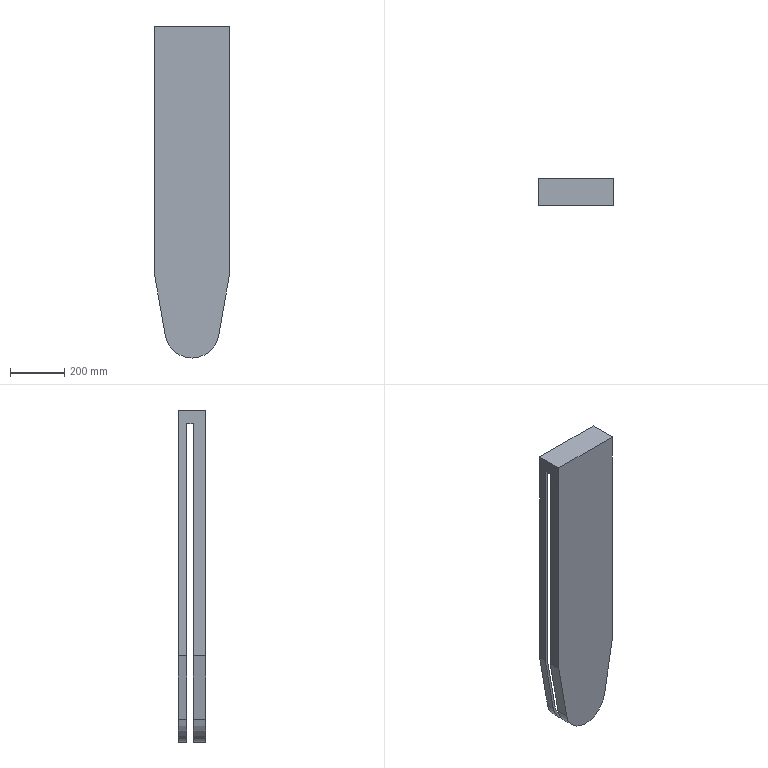Part | SolidWorks | 1 solid | 29 faces | box 280 x 100 x 1224 mm | volume 5139884 mm3 | plane 21 | cylinder 8 | commonest cylinder face diameters 180 x4 200 x4
STEP:
#1=CARTESIAN_POINT('',(88.633,45.,-1139.751));
#2=VERTEX_POINT('',#1);
#3=CARTESIAN_POINT('',(0.,45.,-1214.123));
#4=VERTEX_POINT('',#3);
#5=CARTESIAN_POINT('',(0.,45.,-1124.123));
#6=DIRECTION('',(0.,1.,0.));
#7=DIRECTION('',(0.,0.,-1.));
#8=AXIS2_PLACEMENT_3D('',#5,#6,#7);
#9=CIRCLE('',#8,90.);
#10=EDGE_CURVE('',#2,#4,#9,.T.);
#11=ORIENTED_EDGE('',*,*,#10,.T.);
#12=CARTESIAN_POINT('',(0.,10.,-1214.123));
#13=VERTEX_POINT('',#12);
#14=CARTESIAN_POINT('',(0.,100.,-1214.123));
#15=DIRECTION('',(0.,-1.,0.));
#16=VECTOR('',#15,1000.);
#17=LINE('',#14,#16);
#18=EDGE_CURVE('',#4,#13,#17,.T.);
#19=ORIENTED_EDGE('',*,*,#18,.T.);
#20=CARTESIAN_POINT('',(88.633,10.,-1139.751));
#21=VERTEX_POINT('',#20);
#22=CARTESIAN_POINT('',(0.,10.,-1124.123));
#23=DIRECTION('',(0.,-1.,0.));
#24=DIRECTION('',(0.,0.,-1.));
#25=AXIS2_PLACEMENT_3D('',#22,#23,#24);
#26=CIRCLE('',#25,90.);
#27=EDGE_CURVE('',#13,#21,#26,.T.);
#28=ORIENTED_EDGE('',*,*,#27,.T.);
#29=CARTESIAN_POINT('',(88.633,100.,-1139.751));
#30=DIRECTION('',(0.,1.,0.));
#31=VECTOR('',#30,1000.);
#32=LINE('',#29,#31);
#33=EDGE_CURVE('',#21,#2,#32,.T.);
#34=ORIENTED_EDGE('',*,*,#33,.T.);
#35=EDGE_LOOP('',(#11,#19,#28,#34));
#36=FACE_OUTER_BOUND('',#35,.T.);
#37=CARTESIAN_POINT('',(0.,100.,-1124.123));
#38=DIRECTION('',(0.,-1.,0.));
#39=DIRECTION('',(0.,0.,-1.));
#40=AXIS2_PLACEMENT_3D('',#37,#38,#39);
#41=CYLINDRICAL_SURFACE('',#40,90.);
#42=ADVANCED_FACE('',(#36),#41,.F.);
#43=CARTESIAN_POINT('',(0.,45.,-1224.123));
#44=VERTEX_POINT('',#43);
#45=CARTESIAN_POINT('',(-98.481,45.,-1141.488));
#46=VERTEX_POINT('',#45);
#47=CARTESIAN_POINT('',(0.,45.,-1124.123));
#48=DIRECTION('',(0.,1.,0.));
#49=DIRECTION('',(0.,0.,-1.));
#50=AXIS2_PLACEMENT_3D('',#47,#48,#49);
#51=CIRCLE('',#50,100.);
#52=EDGE_CURVE('',#44,#46,#51,.T.);
#53=ORIENTED_EDGE('',*,*,#52,.F.);
#54=CARTESIAN_POINT('',(0.,0.,-1224.123));
#55=VERTEX_POINT('',#54);
#56=CARTESIAN_POINT('',(0.,100.,-1224.123));
#57=DIRECTION('',(0.,-1.,0.));
#58=VECTOR('',#57,1000.);
#59=LINE('',#56,#58);
#60=EDGE_CURVE('',#44,#55,#59,.T.);
#61=ORIENTED_EDGE('',*,*,#60,.T.);
#62=CARTESIAN_POINT('',(-98.481,0.,-1141.488));
#63=VERTEX_POINT('',#62);
#64=CARTESIAN_POINT('',(0.,0.,-1124.123));
#65=DIRECTION('',(0.,-1.,0.));
#66=DIRECTION('',(0.,0.,-1.));
#67=AXIS2_PLACEMENT_3D('',#64,#65,#66);
#68=CIRCLE('',#67,100.);
#69=EDGE_CURVE('',#63,#55,#68,.T.);
#70=ORIENTED_EDGE('',*,*,#69,.F.);
#71=CARTESIAN_POINT('',(-98.481,100.,-1141.488));
#72=DIRECTION('',(0.,-1.,0.));
#73=VECTOR('',#72,1000.);
#74=LINE('',#71,#73);
#75=EDGE_CURVE('',#46,#63,#74,.T.);
#76=ORIENTED_EDGE('',*,*,#75,.F.);
#77=EDGE_LOOP('',(#53,#61,#70,#76));
#78=FACE_OUTER_BOUND('',#77,.T.);
#79=CARTESIAN_POINT('',(0.,100.,-1124.123));
#80=DIRECTION('',(0.,-1.,0.));
#81=DIRECTION('',(0.,0.,-1.));
#82=AXIS2_PLACEMENT_3D('',#79,#80,#81);
#83=CYLINDRICAL_SURFACE('',#82,100.);
#84=ADVANCED_FACE('',(#78),#83,.T.);
#85=CARTESIAN_POINT('',(88.633,100.,-1139.751));
#86=VERTEX_POINT('',#85);
#87=CARTESIAN_POINT('',(0.,100.,-1214.123));
#88=VERTEX_POINT('',#87);
#89=CARTESIAN_POINT('',(0.,100.,-1124.123));
#90=DIRECTION('',(0.,1.,0.));
#91=DIRECTION('',(0.,0.,-1.));
#92=AXIS2_PLACEMENT_3D('',#89,#90,#91);
#93=CIRCLE('',#92,90.);
#94=EDGE_CURVE('',#86,#88,#93,.T.);
#95=ORIENTED_EDGE('',*,*,#94,.T.);
#96=CARTESIAN_POINT('',(0.,70.,-1214.123));
#97=VERTEX_POINT('',#96);
#98=CARTESIAN_POINT('',(0.,100.,-1214.123));
#99=DIRECTION('',(0.,-1.,0.));
#100=VECTOR('',#99,1000.);
#101=LINE('',#98,#100);
#102=EDGE_CURVE('',#88,#97,#101,.T.);
#103=ORIENTED_EDGE('',*,*,#102,.T.);
#104=CARTESIAN_POINT('',(88.633,70.,-1139.751));
#105=VERTEX_POINT('',#104);
#106=CARTESIAN_POINT('',(0.,70.,-1124.123));
#107=DIRECTION('',(0.,-1.,0.));
#108=DIRECTION('',(0.,0.,1.));
#109=AXIS2_PLACEMENT_3D('',#106,#107,#108);
#110=CIRCLE('',#109,90.);
#111=EDGE_CURVE('',#97,#105,#110,.T.);
#112=ORIENTED_EDGE('',*,*,#111,.T.);
#113=CARTESIAN_POINT('',(88.633,100.,-1139.751));
#114=DIRECTION('',(0.,1.,0.));
#115=VECTOR('',#114,1000.);
#116=LINE('',#113,#115);
#117=EDGE_CURVE('',#105,#86,#116,.T.);
#118=ORIENTED_EDGE('',*,*,#117,.T.);
#119=EDGE_LOOP('',(#95,#103,#112,#118));
#120=FACE_OUTER_BOUND('',#119,.T.);
#121=CARTESIAN_POINT('',(0.,100.,-1124.123));
#122=DIRECTION('',(0.,-1.,0.));
#123=DIRECTION('',(0.,0.,-1.));
#124=AXIS2_PLACEMENT_3D('',#121,#122,#123);
#125=CYLINDRICAL_SURFACE('',#124,90.);
#126=ADVANCED_FACE('',(#120),#125,.F.);
#127=CARTESIAN_POINT('',(0.,100.,-1224.123));
#128=VERTEX_POINT('',#127);
#129=CARTESIAN_POINT('',(-98.481,100.,-1141.488));
#130=VERTEX_POINT('',#129);
#131=CARTESIAN_POINT('',(0.,100.,-1124.123));
#132=DIRECTION('',(0.,1.,0.));
#133=DIRECTION('',(0.,0.,-1.));
#134=AXIS2_PLACEMENT_3D('',#131,#132,#133);
#135=CIRCLE('',#134,100.);
#136=EDGE_CURVE('',#128,#130,#135,.T.);
#137=ORIENTED_EDGE('',*,*,#136,.F.);
#138=CARTESIAN_POINT('',(0.,70.,-1224.123));
#139=VERTEX_POINT('',#138);
#140=CARTESIAN_POINT('',(0.,100.,-1224.123));
#141=DIRECTION('',(0.,-1.,0.));
#142=VECTOR('',#141,1000.);
#143=LINE('',#140,#142);
#144=EDGE_CURVE('',#128,#139,#143,.T.);
#145=ORIENTED_EDGE('',*,*,#144,.T.);
#146=CARTESIAN_POINT('',(-98.481,70.,-1141.488));
#147=VERTEX_POINT('',#146);
#148=CARTESIAN_POINT('',(0.,70.,-1124.123));
#149=DIRECTION('',(0.,-1.,0.));
#150=DIRECTION('',(0.,0.,1.));
#151=AXIS2_PLACEMENT_3D('',#148,#149,#150);
#152=CIRCLE('',#151,100.);
#153=EDGE_CURVE('',#147,#139,#152,.T.);
#154=ORIENTED_EDGE('',*,*,#153,.F.);
#155=CARTESIAN_POINT('',(-98.481,100.,-1141.488));
#156=DIRECTION('',(0.,-1.,0.));
#157=VECTOR('',#156,1000.);
#158=LINE('',#155,#157);
#159=EDGE_CURVE('',#130,#147,#158,.T.);
#160=ORIENTED_EDGE('',*,*,#159,.F.);
#161=EDGE_LOOP('',(#137,#145,#154,#160));
#162=FACE_OUTER_BOUND('',#161,.T.);
#163=CARTESIAN_POINT('',(0.,100.,-1124.123));
#164=DIRECTION('',(0.,-1.,0.));
#165=DIRECTION('',(0.,0.,-1.));
#166=AXIS2_PLACEMENT_3D('',#163,#164,#165);
#167=CYLINDRICAL_SURFACE('',#166,100.);
#168=ADVANCED_FACE('',(#162),#167,.T.);
#169=ORIENTED_EDGE('',*,*,#159,.T.);
#170=CARTESIAN_POINT('',(-140.,70.,-906.021));
#171=VERTEX_POINT('',#170);
#172=CARTESIAN_POINT('',(0.,70.,-1700.));
#173=DIRECTION('',(-0.1736,0.,0.9848));
#174=VECTOR('',#173,1000.);
#175=LINE('',#172,#174);
#176=EDGE_CURVE('',#147,#171,#175,.T.);
#177=ORIENTED_EDGE('',*,*,#176,.T.);
#178=CARTESIAN_POINT('',(-140.,100.,-906.021));
#179=VERTEX_POINT('',#178);
#180=CARTESIAN_POINT('',(-140.,100.,-906.021));
#181=DIRECTION('',(0.,-1.,0.));
#182=VECTOR('',#181,1000.);
#183=LINE('',#180,#182);
#184=EDGE_CURVE('',#179,#171,#183,.T.);
#185=ORIENTED_EDGE('',*,*,#184,.F.);
#186=CARTESIAN_POINT('',(0.,100.,-1700.));
#187=DIRECTION('',(-0.1736,0.,0.9848));
#188=VECTOR('',#187,1000.);
#189=LINE('',#186,#188);
#190=EDGE_CURVE('',#130,#179,#189,.T.);
#191=ORIENTED_EDGE('',*,*,#190,.F.);
#192=EDGE_LOOP('',(#169,#177,#185,#191));
#193=FACE_OUTER_BOUND('',#192,.T.);
#194=CARTESIAN_POINT('',(0.,100.,-1700.));
#195=DIRECTION('',(0.9848,0.,0.1736));
#196=DIRECTION('',(0.1736,0.,-0.9848));
#197=AXIS2_PLACEMENT_3D('',#194,#195,#196);
#198=PLANE('',#197);
#199=ADVANCED_FACE('',(#193),#198,.F.);
#200=CARTESIAN_POINT('',(140.,100.,-906.021));
#201=VERTEX_POINT('',#200);
#202=CARTESIAN_POINT('',(140.,70.,-906.021));
#203=VERTEX_POINT('',#202);
#204=CARTESIAN_POINT('',(140.,100.,-906.021));
#205=DIRECTION('',(0.,-1.,0.));
#206=VECTOR('',#205,1000.);
#207=LINE('',#204,#206);
#208=EDGE_CURVE('',#201,#203,#207,.T.);
#209=ORIENTED_EDGE('',*,*,#208,.T.);
#210=CARTESIAN_POINT('',(98.481,70.,-1141.488));
#211=VERTEX_POINT('',#210);
#212=CARTESIAN_POINT('',(0.,70.,-1700.));
#213=DIRECTION('',(-0.1736,0.,-0.9848));
#214=VECTOR('',#213,1000.);
#215=LINE('',#212,#214);
#216=EDGE_CURVE('',#203,#211,#215,.T.);
#217=ORIENTED_EDGE('',*,*,#216,.T.);
#218=CARTESIAN_POINT('',(98.481,100.,-1141.488));
#219=VERTEX_POINT('',#218);
#220=CARTESIAN_POINT('',(98.481,100.,-1141.488));
#221=DIRECTION('',(0.,1.,0.));
#222=VECTOR('',#221,1000.);
#223=LINE('',#220,#222);
#224=EDGE_CURVE('',#211,#219,#223,.T.);
#225=ORIENTED_EDGE('',*,*,#224,.T.);
#226=CARTESIAN_POINT('',(0.,100.,-1700.));
#227=DIRECTION('',(-0.1736,0.,-0.9848));
#228=VECTOR('',#227,1000.);
#229=LINE('',#226,#228);
#230=EDGE_CURVE('',#201,#219,#229,.T.);
#231=ORIENTED_EDGE('',*,*,#230,.F.);
#232=EDGE_LOOP('',(#209,#217,#225,#231));
#233=FACE_OUTER_BOUND('',#232,.T.);
#234=CARTESIAN_POINT('',(0.,100.,-1700.));
#235=DIRECTION('',(-0.9848,0.,0.1736));
#236=DIRECTION('',(0.1736,0.,0.9848));
#237=AXIS2_PLACEMENT_3D('',#234,#235,#236);
#238=PLANE('',#237);
#239=ADVANCED_FACE('',(#233),#238,.F.);
#240=ORIENTED_EDGE('',*,*,#144,.F.);
#241=CARTESIAN_POINT('',(0.,100.,-1124.123));
#242=DIRECTION('',(0.,1.,0.));
#243=DIRECTION('',(0.,0.,-1.));
#244=AXIS2_PLACEMENT_3D('',#241,#242,#243);
#245=CIRCLE('',#244,100.);
#246=EDGE_CURVE('',#219,#128,#245,.T.);
#247=ORIENTED_EDGE('',*,*,#246,.F.);
#248=ORIENTED_EDGE('',*,*,#224,.F.);
#249=CARTESIAN_POINT('',(0.,70.,-1124.123));
#250=DIRECTION('',(0.,-1.,0.));
#251=DIRECTION('',(0.,0.,1.));
#252=AXIS2_PLACEMENT_3D('',#249,#250,#251);
#253=CIRCLE('',#252,100.);
#254=EDGE_CURVE('',#139,#211,#253,.T.);
#255=ORIENTED_EDGE('',*,*,#254,.F.);
#256=EDGE_LOOP('',(#240,#247,#248,#255));
#257=FACE_OUTER_BOUND('',#256,.T.);
#258=CARTESIAN_POINT('',(0.,100.,-1124.123));
#259=DIRECTION('',(0.,-1.,0.));
#260=DIRECTION('',(0.,0.,-1.));
#261=AXIS2_PLACEMENT_3D('',#258,#259,#260);
#262=CYLINDRICAL_SURFACE('',#261,100.);
#263=ADVANCED_FACE('',(#257),#262,.T.);
#264=CARTESIAN_POINT('',(-88.633,70.,-1139.751));
#265=VERTEX_POINT('',#264);
#266=CARTESIAN_POINT('',(-130.,70.,-905.146));
#267=VERTEX_POINT('',#266);
#268=CARTESIAN_POINT('',(9.848,70.,-1698.264));
#269=DIRECTION('',(-0.1736,0.,0.9848));
#270=VECTOR('',#269,1000.);
#271=LINE('',#268,#270);
#272=EDGE_CURVE('',#265,#267,#271,.T.);
#273=ORIENTED_EDGE('',*,*,#272,.F.);
#274=CARTESIAN_POINT('',(-88.633,100.,-1139.751));
#275=VERTEX_POINT('',#274);
#276=CARTESIAN_POINT('',(-88.633,100.,-1139.751));
#277=DIRECTION('',(0.,-1.,0.));
#278=VECTOR('',#277,1000.);
#279=LINE('',#276,#278);
#280=EDGE_CURVE('',#275,#265,#279,.T.);
#281=ORIENTED_EDGE('',*,*,#280,.F.);
#282=CARTESIAN_POINT('',(-130.,100.,-905.146));
#283=VERTEX_POINT('',#282);
#284=CARTESIAN_POINT('',(-280.869,100.,-49.525));
#285=DIRECTION('',(-0.1736,0.,0.9848));
#286=VECTOR('',#285,1000.);
#287=LINE('',#284,#286);
#288=EDGE_CURVE('',#275,#283,#287,.T.);
#289=ORIENTED_EDGE('',*,*,#288,.T.);
#290=CARTESIAN_POINT('',(-130.,100.,-905.146));
#291=DIRECTION('',(0.,-1.,0.));
#292=VECTOR('',#291,1000.);
#293=LINE('',#290,#292);
#294=EDGE_CURVE('',#283,#267,#293,.T.);
#295=ORIENTED_EDGE('',*,*,#294,.T.);
#296=EDGE_LOOP('',(#273,#281,#289,#295));
#297=FACE_OUTER_BOUND('',#296,.T.);
#298=CARTESIAN_POINT('',(9.848,100.,-1698.264));
#299=DIRECTION('',(0.9848,0.,0.1736));
#300=DIRECTION('',(0.1736,0.,-0.9848));
#301=AXIS2_PLACEMENT_3D('',#298,#299,#300);
#302=PLANE('',#301);
#303=ADVANCED_FACE('',(#297),#302,.T.);
#304=CARTESIAN_POINT('',(130.,70.,-905.146));
#305=VERTEX_POINT('',#304);
#306=CARTESIAN_POINT('',(-9.848,70.,-1698.264));
#307=DIRECTION('',(-0.1736,0.,-0.9848));
#308=VECTOR('',#307,1000.);
#309=LINE('',#306,#308);
#310=EDGE_CURVE('',#305,#105,#309,.T.);
#311=ORIENTED_EDGE('',*,*,#310,.F.);
#312=CARTESIAN_POINT('',(130.,100.,-905.146));
#313=VERTEX_POINT('',#312);
#314=CARTESIAN_POINT('',(130.,100.,-905.146));
#315=DIRECTION('',(0.,-1.,0.));
#316=VECTOR('',#315,1000.);
#317=LINE('',#314,#316);
#318=EDGE_CURVE('',#313,#305,#317,.T.);
#319=ORIENTED_EDGE('',*,*,#318,.F.);
#320=CARTESIAN_POINT('',(280.869,100.,-49.525));
#321=DIRECTION('',(-0.1736,0.,-0.9848));
#322=VECTOR('',#321,1000.);
#323=LINE('',#320,#322);
#324=EDGE_CURVE('',#313,#86,#323,.T.);
#325=ORIENTED_EDGE('',*,*,#324,.T.);
#326=ORIENTED_EDGE('',*,*,#117,.F.);
#327=EDGE_LOOP('',(#311,#319,#325,#326));
#328=FACE_OUTER_BOUND('',#327,.T.);
#329=CARTESIAN_POINT('',(-9.848,100.,-1698.264));
#330=DIRECTION('',(-0.9848,0.,0.1736));
#331=DIRECTION('',(0.1736,0.,0.9848));
#332=AXIS2_PLACEMENT_3D('',#329,#330,#331);
#333=PLANE('',#332);
#334=ADVANCED_FACE('',(#328),#333,.T.);
#335=ORIENTED_EDGE('',*,*,#102,.F.);
#336=CARTESIAN_POINT('',(0.,100.,-1124.123));
#337=DIRECTION('',(0.,1.,0.));
#338=DIRECTION('',(0.,0.,-1.));
#339=AXIS2_PLACEMENT_3D('',#336,#337,#338);
#340=CIRCLE('',#339,90.);
#341=EDGE_CURVE('',#88,#275,#340,.T.);
#342=ORIENTED_EDGE('',*,*,#341,.T.);
#343=ORIENTED_EDGE('',*,*,#280,.T.);
#344=CARTESIAN_POINT('',(0.,70.,-1124.123));
#345=DIRECTION('',(0.,-1.,0.));
#346=DIRECTION('',(0.,0.,1.));
#347=AXIS2_PLACEMENT_3D('',#344,#345,#346);
#348=CIRCLE('',#347,90.);
#349=EDGE_CURVE('',#265,#97,#348,.T.);
#350=ORIENTED_EDGE('',*,*,#349,.T.);
#351=EDGE_LOOP('',(#335,#342,#343,#350));
#352=FACE_OUTER_BOUND('',#351,.T.);
#353=CARTESIAN_POINT('',(0.,100.,-1124.123));
#354=DIRECTION('',(0.,-1.,0.));
#355=DIRECTION('',(0.,0.,-1.));
#356=AXIS2_PLACEMENT_3D('',#353,#354,#355);
#357=CYLINDRICAL_SURFACE('',#356,90.);
#358=ADVANCED_FACE('',(#352),#357,.F.);
#359=ORIENTED_EDGE('',*,*,#230,.T.);
#360=ORIENTED_EDGE('',*,*,#246,.T.);
#361=ORIENTED_EDGE('',*,*,#136,.T.);
#362=ORIENTED_EDGE('',*,*,#190,.T.);
#363=CARTESIAN_POINT('',(-140.,100.,0.));
#364=VERTEX_POINT('',#363);
#365=CARTESIAN_POINT('',(-140.,100.,-906.021));
#366=DIRECTION('',(0.,0.,1.));
#367=VECTOR('',#366,1000.);
#368=LINE('',#365,#367);
#369=EDGE_CURVE('',#179,#364,#368,.T.);
#370=ORIENTED_EDGE('',*,*,#369,.T.);
#371=CARTESIAN_POINT('',(140.,100.,0.));
#372=VERTEX_POINT('',#371);
#373=CARTESIAN_POINT('',(140.,100.,0.));
#374=DIRECTION('',(1.,0.,0.));
#375=VECTOR('',#374,1000.);
#376=LINE('',#373,#375);
#377=EDGE_CURVE('',#364,#372,#376,.T.);
#378=ORIENTED_EDGE('',*,*,#377,.T.);
#379=CARTESIAN_POINT('',(140.,100.,-906.021));
#380=DIRECTION('',(0.,0.,-1.));
#381=VECTOR('',#380,1000.);
#382=LINE('',#379,#381);
#383=EDGE_CURVE('',#372,#201,#382,.T.);
#384=ORIENTED_EDGE('',*,*,#383,.T.);
#385=EDGE_LOOP('',(#359,#360,#361,#362,#370,#378,#384));
#386=FACE_OUTER_BOUND('',#385,.T.);
#387=ORIENTED_EDGE('',*,*,#324,.F.);
#388=CARTESIAN_POINT('',(130.,100.,-10.));
#389=VERTEX_POINT('',#388);
#390=CARTESIAN_POINT('',(130.,100.,0.));
#391=DIRECTION('',(0.,0.,-1.));
#392=VECTOR('',#391,1000.);
#393=LINE('',#390,#392);
#394=EDGE_CURVE('',#389,#313,#393,.T.);
#395=ORIENTED_EDGE('',*,*,#394,.F.);
#396=CARTESIAN_POINT('',(-130.,100.,-10.));
#397=VERTEX_POINT('',#396);
#398=CARTESIAN_POINT('',(0.,100.,-10.));
#399=DIRECTION('',(1.,0.,0.));
#400=VECTOR('',#399,1000.);
#401=LINE('',#398,#400);
#402=EDGE_CURVE('',#397,#389,#401,.T.);
#403=ORIENTED_EDGE('',*,*,#402,.F.);
#404=CARTESIAN_POINT('',(-130.,100.,0.));
#405=DIRECTION('',(0.,0.,1.));
#406=VECTOR('',#405,1000.);
#407=LINE('',#404,#406);
#408=EDGE_CURVE('',#283,#397,#407,.T.);
#409=ORIENTED_EDGE('',*,*,#408,.F.);
#410=ORIENTED_EDGE('',*,*,#288,.F.);
#411=ORIENTED_EDGE('',*,*,#341,.F.);
#412=ORIENTED_EDGE('',*,*,#94,.F.);
#413=EDGE_LOOP('',(#387,#395,#403,#409,#410,#411,#412));
#414=FACE_BOUND('',#413,.T.);
#415=CARTESIAN_POINT('',(0.,100.,0.));
#416=DIRECTION('',(0.,-1.,0.));
#417=DIRECTION('',(0.,0.,-1.));
#418=AXIS2_PLACEMENT_3D('',#415,#416,#417);
#419=PLANE('',#418);
#420=ADVANCED_FACE('',(#386,#414),#419,.F.);
#421=CARTESIAN_POINT('',(-140.,45.,-906.021));
#422=VERTEX_POINT('',#421);
#423=CARTESIAN_POINT('',(-140.,0.,-906.021));
#424=VERTEX_POINT('',#423);
#425=CARTESIAN_POINT('',(-140.,100.,-906.021));
#426=DIRECTION('',(0.,-1.,0.));
#427=VECTOR('',#426,1000.);
#428=LINE('',#425,#427);
#429=EDGE_CURVE('',#422,#424,#428,.T.);
#430=ORIENTED_EDGE('',*,*,#429,.F.);
#431=CARTESIAN_POINT('',(0.,45.,-1700.));
#432=DIRECTION('',(0.1736,0.,-0.9848));
#433=VECTOR('',#432,1000.);
#434=LINE('',#431,#433);
#435=EDGE_CURVE('',#422,#46,#434,.T.);
#436=ORIENTED_EDGE('',*,*,#435,.T.);
#437=ORIENTED_EDGE('',*,*,#75,.T.);
#438=CARTESIAN_POINT('',(0.,0.,-1700.));
#439=DIRECTION('',(-0.1736,0.,0.9848));
#440=VECTOR('',#439,1000.);
#441=LINE('',#438,#440);
#442=EDGE_CURVE('',#63,#424,#441,.T.);
#443=ORIENTED_EDGE('',*,*,#442,.T.);
#444=EDGE_LOOP('',(#430,#436,#437,#443));
#445=FACE_OUTER_BOUND('',#444,.T.);
#446=CARTESIAN_POINT('',(0.,100.,-1700.));
#447=DIRECTION('',(0.9848,0.,0.1736));
#448=DIRECTION('',(0.1736,0.,-0.9848));
#449=AXIS2_PLACEMENT_3D('',#446,#447,#448);
#450=PLANE('',#449);
#451=ADVANCED_FACE('',(#445),#450,.F.);
#452=ORIENTED_EDGE('',*,*,#184,.T.);
#453=CARTESIAN_POINT('',(-140.,70.,-50.));
#454=VERTEX_POINT('',#453);
#455=CARTESIAN_POINT('',(-140.,70.,-1224.123));
#456=DIRECTION('',(0.,0.,-1.));
#457=VECTOR('',#456,1000.);
#458=LINE('',#455,#457);
#459=EDGE_CURVE('',#454,#171,#458,.T.);
#460=ORIENTED_EDGE('',*,*,#459,.F.);
#461=CARTESIAN_POINT('',(-140.,45.,-50.));
#462=VERTEX_POINT('',#461);
#463=CARTESIAN_POINT('',(-140.,70.,-50.));
#464=DIRECTION('',(0.,1.,0.));
#465=VECTOR('',#464,1000.);
#466=LINE('',#463,#465);
#467=EDGE_CURVE('',#462,#454,#466,.T.);
#468=ORIENTED_EDGE('',*,*,#467,.F.);
#469=CARTESIAN_POINT('',(-140.,45.,-1224.123));
#470=DIRECTION('',(0.,0.,1.));
#471=VECTOR('',#470,1000.);
#472=LINE('',#469,#471);
#473=EDGE_CURVE('',#422,#462,#472,.T.);
#474=ORIENTED_EDGE('',*,*,#473,.F.);
#475=ORIENTED_EDGE('',*,*,#429,.T.);
#476=CARTESIAN_POINT('',(-140.,0.,0.));
#477=VERTEX_POINT('',#476);
#478=CARTESIAN_POINT('',(-140.,0.,-906.021));
#479=DIRECTION('',(0.,0.,1.));
#480=VECTOR('',#479,1000.);
#481=LINE('',#478,#480);
#482=EDGE_CURVE('',#424,#477,#481,.T.);
#483=ORIENTED_EDGE('',*,*,#482,.T.);
#484=CARTESIAN_POINT('',(-140.,100.,0.));
#485=DIRECTION('',(0.,-1.,0.));
#486=VECTOR('',#485,1000.);
#487=LINE('',#484,#486);
#488=EDGE_CURVE('',#364,#477,#487,.T.);
#489=ORIENTED_EDGE('',*,*,#488,.F.);
#490=ORIENTED_EDGE('',*,*,#369,.F.);
#491=EDGE_LOOP('',(#452,#460,#468,#474,#475,#483,#489,#490));
#492=FACE_OUTER_BOUND('',#491,.T.);
#493=CARTESIAN_POINT('',(-140.,100.,-906.021));
#494=DIRECTION('',(1.,0.,0.));
#495=DIRECTION('',(0.,0.,-1.));
#496=AXIS2_PLACEMENT_3D('',#493,#494,#495);
#497=PLANE('',#496);
#498=ADVANCED_FACE('',(#492),#497,.F.);
#499=CARTESIAN_POINT('',(140.,0.,0.));
#500=VERTEX_POINT('',#499);
#501=CARTESIAN_POINT('',(140.,0.,0.));
#502=DIRECTION('',(1.,0.,0.));
#503=VECTOR('',#502,1000.);
#504=LINE('',#501,#503);
#505=EDGE_CURVE('',#477,#500,#504,.T.);
#506=ORIENTED_EDGE('',*,*,#505,.T.);
#507=CARTESIAN_POINT('',(140.,100.,0.));
#508=DIRECTION('',(0.,-1.,0.));
#509=VECTOR('',#508,1000.);
#510=LINE('',#507,#509);
#511=EDGE_CURVE('',#372,#500,#510,.T.);
#512=ORIENTED_EDGE('',*,*,#511,.F.);
#513=ORIENTED_EDGE('',*,*,#377,.F.);
#514=ORIENTED_EDGE('',*,*,#488,.T.);
#515=EDGE_LOOP('',(#506,#512,#513,#514));
#516=FACE_OUTER_BOUND('',#515,.T.);
#517=CARTESIAN_POINT('',(140.,100.,0.));
#518=DIRECTION('',(0.,0.,-1.));
#519=DIRECTION('',(-1.,0.,0.));
#520=AXIS2_PLACEMENT_3D('',#517,#518,#519);
#521=PLANE('',#520);
#522=ADVANCED_FACE('',(#516),#521,.F.);
#523=CARTESIAN_POINT('',(140.,45.,-50.));
#524=VERTEX_POINT('',#523);
#525=CARTESIAN_POINT('',(140.,70.,-50.));
#526=VERTEX_POINT('',#525);
#527=CARTESIAN_POINT('',(140.,100.,-50.));
#528=DIRECTION('',(0.,1.,0.));
#529=VECTOR('',#528,1000.);
#530=LINE('',#527,#529);
#531=EDGE_CURVE('',#524,#526,#530,.T.);
#532=ORIENTED_EDGE('',*,*,#531,.T.);
#533=CARTESIAN_POINT('',(140.,70.,-906.021));
#534=DIRECTION('',(0.,0.,-1.));
#535=VECTOR('',#534,1000.);
#536=LINE('',#533,#535);
#537=EDGE_CURVE('',#526,#203,#536,.T.);
#538=ORIENTED_EDGE('',*,*,#537,.T.);
#539=ORIENTED_EDGE('',*,*,#208,.F.);
#540=ORIENTED_EDGE('',*,*,#383,.F.);
#541=ORIENTED_EDGE('',*,*,#511,.T.);
#542=CARTESIAN_POINT('',(140.,0.,-906.021));
#543=VERTEX_POINT('',#542);
#544=CARTESIAN_POINT('',(140.,0.,-906.021));
#545=DIRECTION('',(0.,0.,-1.));
#546=VECTOR('',#545,1000.);
#547=LINE('',#544,#546);
#548=EDGE_CURVE('',#500,#543,#547,.T.);
#549=ORIENTED_EDGE('',*,*,#548,.T.);
#550=CARTESIAN_POINT('',(140.,45.,-906.021));
#551=VERTEX_POINT('',#550);
#552=CARTESIAN_POINT('',(140.,100.,-906.021));
#553=DIRECTION('',(0.,-1.,0.));
#554=VECTOR('',#553,1000.);
#555=LINE('',#552,#554);
#556=EDGE_CURVE('',#551,#543,#555,.T.);
#557=ORIENTED_EDGE('',*,*,#556,.F.);
#558=CARTESIAN_POINT('',(140.,45.,-906.021));
#559=DIRECTION('',(0.,0.,1.));
#560=VECTOR('',#559,1000.);
#561=LINE('',#558,#560);
#562=EDGE_CURVE('',#551,#524,#561,.T.);
#563=ORIENTED_EDGE('',*,*,#562,.T.);
#564=EDGE_LOOP('',(#532,#538,#539,#540,#541,#549,#557,#563));
#565=FACE_OUTER_BOUND('',#564,.T.);
#566=CARTESIAN_POINT('',(140.,100.,-906.021));
#567=DIRECTION('',(-1.,0.,0.));
#568=DIRECTION('',(0.,0.,1.));
#569=AXIS2_PLACEMENT_3D('',#566,#567,#568);
#570=PLANE('',#569);
#571=ADVANCED_FACE('',(#565),#570,.F.);
#572=CARTESIAN_POINT('',(98.481,0.,-1141.488));
#573=VERTEX_POINT('',#572);
#574=CARTESIAN_POINT('',(98.481,45.,-1141.488));
#575=VERTEX_POINT('',#574);
#576=CARTESIAN_POINT('',(98.481,100.,-1141.488));
#577=DIRECTION('',(0.,1.,0.));
#578=VECTOR('',#577,1000.);
#579=LINE('',#576,#578);
#580=EDGE_CURVE('',#573,#575,#579,.T.);
#581=ORIENTED_EDGE('',*,*,#580,.T.);
#582=CARTESIAN_POINT('',(0.,45.,-1700.));
#583=DIRECTION('',(0.1736,0.,0.9848));
#584=VECTOR('',#583,1000.);
#585=LINE('',#582,#584);
#586=EDGE_CURVE('',#575,#551,#585,.T.);
#587=ORIENTED_EDGE('',*,*,#586,.T.);
#588=ORIENTED_EDGE('',*,*,#556,.T.);
#589=CARTESIAN_POINT('',(0.,0.,-1700.));
#590=DIRECTION('',(-0.1736,0.,-0.9848));
#591=VECTOR('',#590,1000.);
#592=LINE('',#589,#591);
#593=EDGE_CURVE('',#543,#573,#592,.T.);
#594=ORIENTED_EDGE('',*,*,#593,.T.);
#595=EDGE_LOOP('',(#581,#587,#588,#594));
#596=FACE_OUTER_BOUND('',#595,.T.);
#597=CARTESIAN_POINT('',(0.,100.,-1700.));
#598=DIRECTION('',(-0.9848,0.,0.1736));
#599=DIRECTION('',(0.1736,0.,0.9848));
#600=AXIS2_PLACEMENT_3D('',#597,#598,#599);
#601=PLANE('',#600);
#602=ADVANCED_FACE('',(#596),#601,.F.);
#603=ORIENTED_EDGE('',*,*,#442,.F.);
#604=ORIENTED_EDGE('',*,*,#69,.T.);
#605=CARTESIAN_POINT('',(0.,0.,-1124.123));
#606=DIRECTION('',(0.,-1.,0.));
#607=DIRECTION('',(0.,0.,-1.));
#608=AXIS2_PLACEMENT_3D('',#605,#606,#607);
#609=CIRCLE('',#608,100.);
#610=EDGE_CURVE('',#55,#573,#609,.T.);
#611=ORIENTED_EDGE('',*,*,#610,.T.);
#612=ORIENTED_EDGE('',*,*,#593,.F.);
#613=ORIENTED_EDGE('',*,*,#548,.F.);
#614=ORIENTED_EDGE('',*,*,#505,.F.);
#615=ORIENTED_EDGE('',*,*,#482,.F.);
#616=EDGE_LOOP('',(#603,#604,#611,#612,#613,#614,#615));
#617=FACE_OUTER_BOUND('',#616,.T.);
#618=CARTESIAN_POINT('',(0.,0.,0.));
#619=DIRECTION('',(0.,-1.,0.));
#620=DIRECTION('',(0.,0.,-1.));
#621=AXIS2_PLACEMENT_3D('',#618,#619,#620);
#622=PLANE('',#621);
#623=ADVANCED_FACE('',(#617),#622,.T.);
#624=ORIENTED_EDGE('',*,*,#60,.F.);
#625=CARTESIAN_POINT('',(0.,45.,-1124.123));
#626=DIRECTION('',(0.,1.,0.));
#627=DIRECTION('',(0.,0.,-1.));
#628=AXIS2_PLACEMENT_3D('',#625,#626,#627);
#629=CIRCLE('',#628,100.);
#630=EDGE_CURVE('',#575,#44,#629,.T.);
#631=ORIENTED_EDGE('',*,*,#630,.F.);
#632=ORIENTED_EDGE('',*,*,#580,.F.);
#633=ORIENTED_EDGE('',*,*,#610,.F.);
#634=EDGE_LOOP('',(#624,#631,#632,#633));
#635=FACE_OUTER_BOUND('',#634,.T.);
#636=CARTESIAN_POINT('',(0.,100.,-1124.123));
#637=DIRECTION('',(0.,-1.,0.));
#638=DIRECTION('',(0.,0.,-1.));
#639=AXIS2_PLACEMENT_3D('',#636,#637,#638);
#640=CYLINDRICAL_SURFACE('',#639,100.);
#641=ADVANCED_FACE('',(#635),#640,.T.);
#642=CARTESIAN_POINT('',(-130.,45.,-905.146));
#643=VERTEX_POINT('',#642);
#644=CARTESIAN_POINT('',(-88.633,45.,-1139.751));
#645=VERTEX_POINT('',#644);
#646=CARTESIAN_POINT('',(9.848,45.,-1698.264));
#647=DIRECTION('',(0.1736,0.,-0.9848));
#648=VECTOR('',#647,1000.);
#649=LINE('',#646,#648);
#650=EDGE_CURVE('',#643,#645,#649,.T.);
#651=ORIENTED_EDGE('',*,*,#650,.F.);
#652=CARTESIAN_POINT('',(-130.,10.,-905.146));
#653=VERTEX_POINT('',#652);
#654=CARTESIAN_POINT('',(-130.,100.,-905.146));
#655=DIRECTION('',(0.,-1.,0.));
#656=VECTOR('',#655,1000.);
#657=LINE('',#654,#656);
#658=EDGE_CURVE('',#643,#653,#657,.T.);
#659=ORIENTED_EDGE('',*,*,#658,.T.);
#660=CARTESIAN_POINT('',(-88.633,10.,-1139.751));
#661=VERTEX_POINT('',#660);
#662=CARTESIAN_POINT('',(-280.869,10.,-49.525));
#663=DIRECTION('',(-0.1736,0.,0.9848));
#664=VECTOR('',#663,1000.);
#665=LINE('',#662,#664);
#666=EDGE_CURVE('',#661,#653,#665,.T.);
#667=ORIENTED_EDGE('',*,*,#666,.F.);
#668=CARTESIAN_POINT('',(-88.633,100.,-1139.751));
#669=DIRECTION('',(0.,-1.,0.));
#670=VECTOR('',#669,1000.);
#671=LINE('',#668,#670);
#672=EDGE_CURVE('',#645,#661,#671,.T.);
#673=ORIENTED_EDGE('',*,*,#672,.F.);
#674=EDGE_LOOP('',(#651,#659,#667,#673));
#675=FACE_OUTER_BOUND('',#674,.T.);
#676=CARTESIAN_POINT('',(9.848,100.,-1698.264));
#677=DIRECTION('',(0.9848,0.,0.1736));
#678=DIRECTION('',(0.1736,0.,-0.9848));
#679=AXIS2_PLACEMENT_3D('',#676,#677,#678);
#680=PLANE('',#679);
#681=ADVANCED_FACE('',(#675),#680,.T.);
#682=CARTESIAN_POINT('',(-130.,70.,-50.));
#683=VERTEX_POINT('',#682);
#684=CARTESIAN_POINT('',(-130.,70.,-906.021));
#685=DIRECTION('',(0.,0.,1.));
#686=VECTOR('',#685,1000.);
#687=LINE('',#684,#686);
#688=EDGE_CURVE('',#267,#683,#687,.T.);
#689=ORIENTED_EDGE('',*,*,#688,.F.);
#690=ORIENTED_EDGE('',*,*,#294,.F.);
#691=ORIENTED_EDGE('',*,*,#408,.T.);
#692=CARTESIAN_POINT('',(-130.,10.,-10.));
#693=VERTEX_POINT('',#692);
#694=CARTESIAN_POINT('',(-130.,100.,-10.));
#695=DIRECTION('',(0.,-1.,0.));
#696=VECTOR('',#695,1000.);
#697=LINE('',#694,#696);
#698=EDGE_CURVE('',#397,#693,#697,.T.);
#699=ORIENTED_EDGE('',*,*,#698,.T.);
#700=CARTESIAN_POINT('',(-130.,10.,0.));
#701=DIRECTION('',(0.,0.,1.));
#702=VECTOR('',#701,1000.);
#703=LINE('',#700,#702);
#704=EDGE_CURVE('',#653,#693,#703,.T.);
#705=ORIENTED_EDGE('',*,*,#704,.F.);
#706=ORIENTED_EDGE('',*,*,#658,.F.);
#707=CARTESIAN_POINT('',(-130.,45.,-50.));
#708=VERTEX_POINT('',#707);
#709=CARTESIAN_POINT('',(-130.,45.,-906.021));
#710=DIRECTION('',(0.,0.,-1.));
#711=VECTOR('',#710,1000.);
#712=LINE('',#709,#711);
#713=EDGE_CURVE('',#708,#643,#712,.T.);
#714=ORIENTED_EDGE('',*,*,#713,.F.);
#715=CARTESIAN_POINT('',(-130.,100.,-50.));
#716=DIRECTION('',(0.,-1.,0.));
#717=VECTOR('',#716,1000.);
#718=LINE('',#715,#717);
#719=EDGE_CURVE('',#683,#708,#718,.T.);
#720=ORIENTED_EDGE('',*,*,#719,.F.);
#721=EDGE_LOOP('',(#689,#690,#691,#699,#705,#706,#714,#720));
#722=FACE_OUTER_BOUND('',#721,.T.);
#723=CARTESIAN_POINT('',(-130.,100.,-906.021));
#724=DIRECTION('',(1.,0.,0.));
#725=DIRECTION('',(0.,0.,-1.));
#726=AXIS2_PLACEMENT_3D('',#723,#724,#725);
#727=PLANE('',#726);
#728=ADVANCED_FACE('',(#722),#727,.T.);
#729=CARTESIAN_POINT('',(130.,10.,-10.));
#730=VERTEX_POINT('',#729);
#731=CARTESIAN_POINT('',(0.,10.,-10.));
#732=DIRECTION('',(1.,0.,0.));
#733=VECTOR('',#732,1000.);
#734=LINE('',#731,#733);
#735=EDGE_CURVE('',#693,#730,#734,.T.);
#736=ORIENTED_EDGE('',*,*,#735,.F.);
#737=ORIENTED_EDGE('',*,*,#698,.F.);
#738=ORIENTED_EDGE('',*,*,#402,.T.);
#739=CARTESIAN_POINT('',(130.,100.,-10.));
#740=DIRECTION('',(0.,-1.,0.));
#741=VECTOR('',#740,1000.);
#742=LINE('',#739,#741);
#743=EDGE_CURVE('',#389,#730,#742,.T.);
#744=ORIENTED_EDGE('',*,*,#743,.T.);
#745=EDGE_LOOP('',(#736,#737,#738,#744));
#746=FACE_OUTER_BOUND('',#745,.T.);
#747=CARTESIAN_POINT('',(140.,100.,-10.));
#748=DIRECTION('',(0.,0.,-1.));
#749=DIRECTION('',(-1.,0.,0.));
#750=AXIS2_PLACEMENT_3D('',#747,#748,#749);
#751=PLANE('',#750);
#752=ADVANCED_FACE('',(#746),#751,.T.);
#753=CARTESIAN_POINT('',(130.,70.,-50.));
#754=VERTEX_POINT('',#753);
#755=CARTESIAN_POINT('',(130.,70.,-906.021));
#756=DIRECTION('',(0.,0.,-1.));
#757=VECTOR('',#756,1000.);
#758=LINE('',#755,#757);
#759=EDGE_CURVE('',#754,#305,#758,.T.);
#760=ORIENTED_EDGE('',*,*,#759,.F.);
#761=CARTESIAN_POINT('',(130.,45.,-50.));
#762=VERTEX_POINT('',#761);
#763=CARTESIAN_POINT('',(130.,100.,-50.));
#764=DIRECTION('',(0.,1.,0.));
#765=VECTOR('',#764,1000.);
#766=LINE('',#763,#765);
#767=EDGE_CURVE('',#762,#754,#766,.T.);
#768=ORIENTED_EDGE('',*,*,#767,.F.);
#769=CARTESIAN_POINT('',(130.,45.,-905.146));
#770=VERTEX_POINT('',#769);
#771=CARTESIAN_POINT('',(130.,45.,-906.021));
#772=DIRECTION('',(0.,0.,1.));
#773=VECTOR('',#772,1000.);
#774=LINE('',#771,#773);
#775=EDGE_CURVE('',#770,#762,#774,.T.);
#776=ORIENTED_EDGE('',*,*,#775,.F.);
#777=CARTESIAN_POINT('',(130.,10.,-905.146));
#778=VERTEX_POINT('',#777);
#779=CARTESIAN_POINT('',(130.,100.,-905.146));
#780=DIRECTION('',(0.,-1.,0.));
#781=VECTOR('',#780,1000.);
#782=LINE('',#779,#781);
#783=EDGE_CURVE('',#770,#778,#782,.T.);
#784=ORIENTED_EDGE('',*,*,#783,.T.);
#785=CARTESIAN_POINT('',(130.,10.,0.));
#786=DIRECTION('',(0.,0.,-1.));
#787=VECTOR('',#786,1000.);
#788=LINE('',#785,#787);
#789=EDGE_CURVE('',#730,#778,#788,.T.);
#790=ORIENTED_EDGE('',*,*,#789,.F.);
#791=ORIENTED_EDGE('',*,*,#743,.F.);
#792=ORIENTED_EDGE('',*,*,#394,.T.);
#793=ORIENTED_EDGE('',*,*,#318,.T.);
#794=EDGE_LOOP('',(#760,#768,#776,#784,#790,#791,#792,#793));
#795=FACE_OUTER_BOUND('',#794,.T.);
#796=CARTESIAN_POINT('',(130.,100.,-906.021));
#797=DIRECTION('',(-1.,0.,0.));
#798=DIRECTION('',(0.,0.,1.));
#799=AXIS2_PLACEMENT_3D('',#796,#797,#798);
#800=PLANE('',#799);
#801=ADVANCED_FACE('',(#795),#800,.T.);
#802=CARTESIAN_POINT('',(-9.848,45.,-1698.264));
#803=DIRECTION('',(0.1736,0.,0.9848));
#804=VECTOR('',#803,1000.);
#805=LINE('',#802,#804);
#806=EDGE_CURVE('',#2,#770,#805,.T.);
#807=ORIENTED_EDGE('',*,*,#806,.F.);
#808=ORIENTED_EDGE('',*,*,#33,.F.);
#809=CARTESIAN_POINT('',(280.869,10.,-49.525));
#810=DIRECTION('',(-0.1736,0.,-0.9848));
#811=VECTOR('',#810,1000.);
#812=LINE('',#809,#811);
#813=EDGE_CURVE('',#778,#21,#812,.T.);
#814=ORIENTED_EDGE('',*,*,#813,.F.);
#815=ORIENTED_EDGE('',*,*,#783,.F.);
#816=EDGE_LOOP('',(#807,#808,#814,#815));
#817=FACE_OUTER_BOUND('',#816,.T.);
#818=CARTESIAN_POINT('',(-9.848,100.,-1698.264));
#819=DIRECTION('',(-0.9848,0.,0.1736));
#820=DIRECTION('',(0.1736,0.,0.9848));
#821=AXIS2_PLACEMENT_3D('',#818,#819,#820);
#822=PLANE('',#821);
#823=ADVANCED_FACE('',(#817),#822,.T.);
#824=ORIENTED_EDGE('',*,*,#666,.T.);
#825=ORIENTED_EDGE('',*,*,#704,.T.);
#826=ORIENTED_EDGE('',*,*,#735,.T.);
#827=ORIENTED_EDGE('',*,*,#789,.T.);
#828=ORIENTED_EDGE('',*,*,#813,.T.);
#829=ORIENTED_EDGE('',*,*,#27,.F.);
#830=CARTESIAN_POINT('',(0.,10.,-1124.123));
#831=DIRECTION('',(0.,-1.,0.));
#832=DIRECTION('',(0.,0.,-1.));
#833=AXIS2_PLACEMENT_3D('',#830,#831,#832);
#834=CIRCLE('',#833,90.);
#835=EDGE_CURVE('',#661,#13,#834,.T.);
#836=ORIENTED_EDGE('',*,*,#835,.F.);
#837=EDGE_LOOP('',(#824,#825,#826,#827,#828,#829,#836));
#838=FACE_OUTER_BOUND('',#837,.T.);
#839=CARTESIAN_POINT('',(0.,10.,0.));
#840=DIRECTION('',(0.,-1.,0.));
#841=DIRECTION('',(0.,0.,-1.));
#842=AXIS2_PLACEMENT_3D('',#839,#840,#841);
#843=PLANE('',#842);
#844=ADVANCED_FACE('',(#838),#843,.F.);
#845=ORIENTED_EDGE('',*,*,#18,.F.);
#846=CARTESIAN_POINT('',(0.,45.,-1124.123));
#847=DIRECTION('',(0.,1.,0.));
#848=DIRECTION('',(0.,0.,-1.));
#849=AXIS2_PLACEMENT_3D('',#846,#847,#848);
#850=CIRCLE('',#849,90.);
#851=EDGE_CURVE('',#4,#645,#850,.T.);
#852=ORIENTED_EDGE('',*,*,#851,.T.);
#853=ORIENTED_EDGE('',*,*,#672,.T.);
#854=ORIENTED_EDGE('',*,*,#835,.T.);
#855=EDGE_LOOP('',(#845,#852,#853,#854));
#856=FACE_OUTER_BOUND('',#855,.T.);
#857=CARTESIAN_POINT('',(0.,100.,-1124.123));
#858=DIRECTION('',(0.,-1.,0.));
#859=DIRECTION('',(0.,0.,-1.));
#860=AXIS2_PLACEMENT_3D('',#857,#858,#859);
#861=CYLINDRICAL_SURFACE('',#860,90.);
#862=ADVANCED_FACE('',(#856),#861,.F.);
#863=CARTESIAN_POINT('',(321.,45.,-50.));
#864=DIRECTION('',(-1.,0.,0.));
#865=VECTOR('',#864,1000.);
#866=LINE('',#863,#865);
#867=EDGE_CURVE('',#524,#762,#866,.T.);
#868=ORIENTED_EDGE('',*,*,#867,.T.);
#869=ORIENTED_EDGE('',*,*,#767,.T.);
#870=CARTESIAN_POINT('',(321.,70.,-50.));
#871=DIRECTION('',(-1.,0.,0.));
#872=VECTOR('',#871,1000.);
#873=LINE('',#870,#872);
#874=EDGE_CURVE('',#526,#754,#873,.T.);
#875=ORIENTED_EDGE('',*,*,#874,.F.);
#876=ORIENTED_EDGE('',*,*,#531,.F.);
#877=EDGE_LOOP('',(#868,#869,#875,#876));
#878=FACE_OUTER_BOUND('',#877,.T.);
#879=CARTESIAN_POINT('',(321.,70.,-50.));
#880=DIRECTION('',(0.,0.,1.));
#881=DIRECTION('',(0.,-1.,0.));
#882=AXIS2_PLACEMENT_3D('',#879,#880,#881);
#883=PLANE('',#882);
#884=ADVANCED_FACE('',(#878),#883,.F.);
#885=ORIENTED_EDGE('',*,*,#719,.T.);
#886=CARTESIAN_POINT('',(321.,45.,-50.));
#887=DIRECTION('',(-1.,0.,0.));
#888=VECTOR('',#887,1000.);
#889=LINE('',#886,#888);
#890=EDGE_CURVE('',#708,#462,#889,.T.);
#891=ORIENTED_EDGE('',*,*,#890,.T.);
#892=ORIENTED_EDGE('',*,*,#467,.T.);
#893=CARTESIAN_POINT('',(321.,70.,-50.));
#894=DIRECTION('',(-1.,0.,0.));
#895=VECTOR('',#894,1000.);
#896=LINE('',#893,#895);
#897=EDGE_CURVE('',#683,#454,#896,.T.);
#898=ORIENTED_EDGE('',*,*,#897,.F.);
#899=EDGE_LOOP('',(#885,#891,#892,#898));
#900=FACE_OUTER_BOUND('',#899,.T.);
#901=CARTESIAN_POINT('',(321.,70.,-50.));
#902=DIRECTION('',(0.,0.,1.));
#903=DIRECTION('',(0.,-1.,0.));
#904=AXIS2_PLACEMENT_3D('',#901,#902,#903);
#905=PLANE('',#904);
#906=ADVANCED_FACE('',(#900),#905,.F.);
#907=ORIENTED_EDGE('',*,*,#153,.T.);
#908=ORIENTED_EDGE('',*,*,#254,.T.);
#909=ORIENTED_EDGE('',*,*,#216,.F.);
#910=ORIENTED_EDGE('',*,*,#537,.F.);
#911=ORIENTED_EDGE('',*,*,#874,.T.);
#912=ORIENTED_EDGE('',*,*,#759,.T.);
#913=ORIENTED_EDGE('',*,*,#310,.T.);
#914=ORIENTED_EDGE('',*,*,#111,.F.);
#915=ORIENTED_EDGE('',*,*,#349,.F.);
#916=ORIENTED_EDGE('',*,*,#272,.T.);
#917=ORIENTED_EDGE('',*,*,#688,.T.);
#918=ORIENTED_EDGE('',*,*,#897,.T.);
#919=ORIENTED_EDGE('',*,*,#459,.T.);
#920=ORIENTED_EDGE('',*,*,#176,.F.);
#921=EDGE_LOOP('',(#907,#908,#909,#910,#911,#912,#913,#914,#915,#916,#917,#918,#919,#920));
#922=FACE_OUTER_BOUND('',#921,.T.);
#923=CARTESIAN_POINT('',(321.,70.,-1224.123));
#924=DIRECTION('',(0.,1.,0.));
#925=DIRECTION('',(0.,0.,1.));
#926=AXIS2_PLACEMENT_3D('',#923,#924,#925);
#927=PLANE('',#926);
#928=ADVANCED_FACE('',(#922),#927,.F.);
#929=ORIENTED_EDGE('',*,*,#473,.T.);
#930=ORIENTED_EDGE('',*,*,#890,.F.);
#931=ORIENTED_EDGE('',*,*,#713,.T.);
#932=ORIENTED_EDGE('',*,*,#650,.T.);
#933=ORIENTED_EDGE('',*,*,#851,.F.);
#934=ORIENTED_EDGE('',*,*,#10,.F.);
#935=ORIENTED_EDGE('',*,*,#806,.T.);
#936=ORIENTED_EDGE('',*,*,#775,.T.);
#937=ORIENTED_EDGE('',*,*,#867,.F.);
#938=ORIENTED_EDGE('',*,*,#562,.F.);
#939=ORIENTED_EDGE('',*,*,#586,.F.);
#940=ORIENTED_EDGE('',*,*,#630,.T.);
#941=ORIENTED_EDGE('',*,*,#52,.T.);
#942=ORIENTED_EDGE('',*,*,#435,.F.);
#943=EDGE_LOOP('',(#929,#930,#931,#932,#933,#934,#935,#936,#937,#938,#939,#940,#941,#942));
#944=FACE_OUTER_BOUND('',#943,.T.);
#945=CARTESIAN_POINT('',(321.,45.,-1224.123));
#946=DIRECTION('',(0.,-1.,0.));
#947=DIRECTION('',(0.,0.,-1.));
#948=AXIS2_PLACEMENT_3D('',#945,#946,#947);
#949=PLANE('',#948);
#950=ADVANCED_FACE('',(#944),#949,.F.);
#951=CLOSED_SHELL('',(#42,#84,#126,#168,#199,#239,#263,#303,#334,#358,#420,#451,#498,#522,#571,#602,#623,#641,#681,#728,#752,#801,#823,#844,#862,#884,#906,#928,#950));
#952=MANIFOLD_SOLID_BREP('',#951);
#953=CARTESIAN_POINT('',(0.,0.,0.));
#954=DIRECTION('',(0.,0.,1.));
#955=DIRECTION('',(1.,0.,0.));
#956=AXIS2_PLACEMENT_3D('',#953,#954,#955);
#957=(LENGTH_UNIT()NAMED_UNIT(*)SI_UNIT(.MILLI.,.METRE.));
#958=UNCERTAINTY_MEASURE_WITH_UNIT(LENGTH_MEASURE(0.00001),#957,'','');
#959=(NAMED_UNIT(*)PLANE_ANGLE_UNIT()SI_UNIT($,.RADIAN.));
#960=(NAMED_UNIT(*)SI_UNIT($,.STERADIAN.)SOLID_ANGLE_UNIT());
#961=(GEOMETRIC_REPRESENTATION_CONTEXT(3)GLOBAL_UNCERTAINTY_ASSIGNED_CONTEXT((#958))GLOBAL_UNIT_ASSIGNED_CONTEXT((#957,#959,#960))REPRESENTATION_CONTEXT('',''));
#962=ADVANCED_BREP_SHAPE_REPRESENTATION('',(#952,#956),#961);